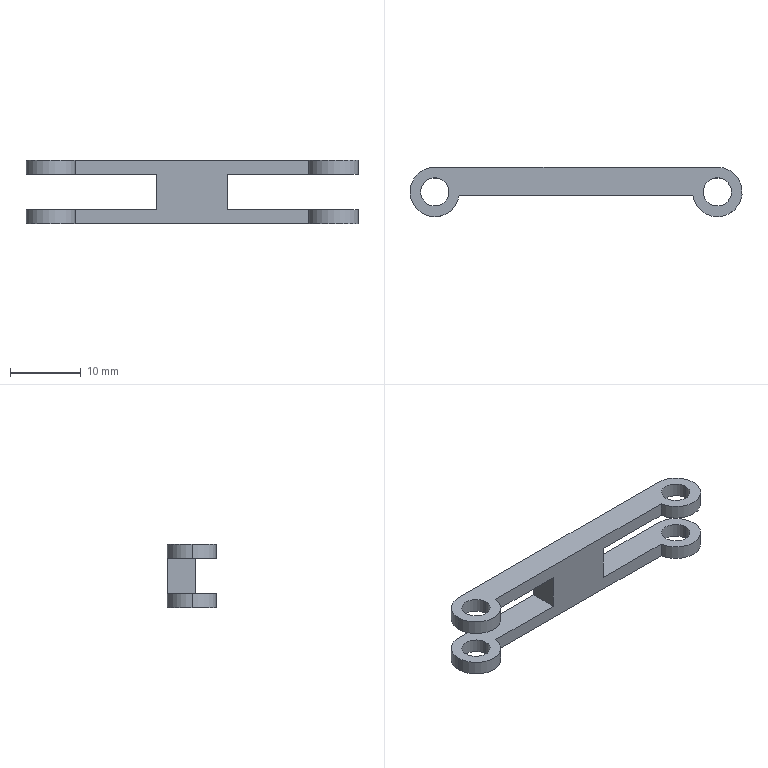Part | SolidWorks | features Extrusion 1, ICE 1, MirrorPattern 1 | 1 solid | 24 faces | box 47 x 7 x 9 mm | volume 956.424 mm3 | cylinder 14 | plane 10 | commonest cylinder face diameters 4 x8 7 x6
STEP:
#1=CARTESIAN_POINT('',(-18.,-3.5,2.));
#2=VERTEX_POINT('',#1);
#3=CARTESIAN_POINT('',(-22.,-3.5,2.));
#4=VERTEX_POINT('',#3);
#5=CARTESIAN_POINT('',(-20.,-3.5,2.));
#6=DIRECTION('',(0.,0.,-1.));
#7=DIRECTION('',(-1.,0.,0.));
#8=AXIS2_PLACEMENT_3D('',#5,#6,#7);
#9=CIRCLE('',#8,2.);
#10=EDGE_CURVE('',#2,#4,#9,.T.);
#11=ORIENTED_EDGE('',*,*,#10,.F.);
#12=CARTESIAN_POINT('',(-18.,-3.5,0.));
#13=VERTEX_POINT('',#12);
#14=CARTESIAN_POINT('',(-18.,-3.5,9.));
#15=DIRECTION('',(0.,0.,-1.));
#16=VECTOR('',#15,1000.);
#17=LINE('',#14,#16);
#18=EDGE_CURVE('',#2,#13,#17,.T.);
#19=ORIENTED_EDGE('',*,*,#18,.T.);
#20=CARTESIAN_POINT('',(-22.,-3.5,0.));
#21=VERTEX_POINT('',#20);
#22=CARTESIAN_POINT('',(-20.,-3.5,0.));
#23=DIRECTION('',(0.,0.,1.));
#24=DIRECTION('',(1.,0.,0.));
#25=AXIS2_PLACEMENT_3D('',#22,#23,#24);
#26=CIRCLE('',#25,2.);
#27=EDGE_CURVE('',#21,#13,#26,.T.);
#28=ORIENTED_EDGE('',*,*,#27,.F.);
#29=CARTESIAN_POINT('',(-22.,-3.5,9.));
#30=DIRECTION('',(0.,0.,-1.));
#31=VECTOR('',#30,1000.);
#32=LINE('',#29,#31);
#33=EDGE_CURVE('',#4,#21,#32,.T.);
#34=ORIENTED_EDGE('',*,*,#33,.F.);
#35=EDGE_LOOP('',(#11,#19,#28,#34));
#36=FACE_OUTER_BOUND('',#35,.T.);
#37=CARTESIAN_POINT('',(-20.,-3.5,9.));
#38=DIRECTION('',(0.,0.,-1.));
#39=DIRECTION('',(-1.,0.,0.));
#40=AXIS2_PLACEMENT_3D('',#37,#38,#39);
#41=CYLINDRICAL_SURFACE('',#40,2.);
#42=ADVANCED_FACE('',(#36),#41,.F.);
#43=CARTESIAN_POINT('',(-16.536,-4.,2.));
#44=VERTEX_POINT('',#43);
#45=CARTESIAN_POINT('',(-23.5,-3.5,2.));
#46=VERTEX_POINT('',#45);
#47=CARTESIAN_POINT('',(-20.,-3.5,2.));
#48=DIRECTION('',(0.,0.,-1.));
#49=DIRECTION('',(-1.,0.,0.));
#50=AXIS2_PLACEMENT_3D('',#47,#48,#49);
#51=CIRCLE('',#50,3.5);
#52=EDGE_CURVE('',#44,#46,#51,.T.);
#53=ORIENTED_EDGE('',*,*,#52,.T.);
#54=CARTESIAN_POINT('',(-23.5,-3.5,0.));
#55=VERTEX_POINT('',#54);
#56=CARTESIAN_POINT('',(-23.5,-3.5,9.));
#57=DIRECTION('',(0.,0.,-1.));
#58=VECTOR('',#57,1000.);
#59=LINE('',#56,#58);
#60=EDGE_CURVE('',#46,#55,#59,.T.);
#61=ORIENTED_EDGE('',*,*,#60,.T.);
#62=CARTESIAN_POINT('',(-16.536,-4.,0.));
#63=VERTEX_POINT('',#62);
#64=CARTESIAN_POINT('',(-20.,-3.5,0.));
#65=DIRECTION('',(0.,0.,1.));
#66=DIRECTION('',(1.,0.,0.));
#67=AXIS2_PLACEMENT_3D('',#64,#65,#66);
#68=CIRCLE('',#67,3.5);
#69=EDGE_CURVE('',#55,#63,#68,.T.);
#70=ORIENTED_EDGE('',*,*,#69,.T.);
#71=CARTESIAN_POINT('',(-16.536,-4.,9.));
#72=DIRECTION('',(0.,0.,-1.));
#73=VECTOR('',#72,1000.);
#74=LINE('',#71,#73);
#75=EDGE_CURVE('',#44,#63,#74,.T.);
#76=ORIENTED_EDGE('',*,*,#75,.F.);
#77=EDGE_LOOP('',(#53,#61,#70,#76));
#78=FACE_OUTER_BOUND('',#77,.T.);
#79=CARTESIAN_POINT('',(-20.,-3.5,9.));
#80=DIRECTION('',(0.,0.,-1.));
#81=DIRECTION('',(-1.,0.,0.));
#82=AXIS2_PLACEMENT_3D('',#79,#80,#81);
#83=CYLINDRICAL_SURFACE('',#82,3.5);
#84=ADVANCED_FACE('',(#78),#83,.T.);
#85=CARTESIAN_POINT('',(-22.,-3.5,9.));
#86=VERTEX_POINT('',#85);
#87=CARTESIAN_POINT('',(-18.,-3.5,9.));
#88=VERTEX_POINT('',#87);
#89=CARTESIAN_POINT('',(-20.,-3.5,9.));
#90=DIRECTION('',(0.,0.,1.));
#91=DIRECTION('',(1.,0.,0.));
#92=AXIS2_PLACEMENT_3D('',#89,#90,#91);
#93=CIRCLE('',#92,2.);
#94=EDGE_CURVE('',#86,#88,#93,.T.);
#95=ORIENTED_EDGE('',*,*,#94,.T.);
#96=CARTESIAN_POINT('',(-18.,-3.5,7.));
#97=VERTEX_POINT('',#96);
#98=CARTESIAN_POINT('',(-18.,-3.5,9.));
#99=DIRECTION('',(0.,0.,-1.));
#100=VECTOR('',#99,1000.);
#101=LINE('',#98,#100);
#102=EDGE_CURVE('',#88,#97,#101,.T.);
#103=ORIENTED_EDGE('',*,*,#102,.T.);
#104=CARTESIAN_POINT('',(-22.,-3.5,7.));
#105=VERTEX_POINT('',#104);
#106=CARTESIAN_POINT('',(-20.,-3.5,7.));
#107=DIRECTION('',(0.,0.,1.));
#108=DIRECTION('',(1.,0.,0.));
#109=AXIS2_PLACEMENT_3D('',#106,#107,#108);
#110=CIRCLE('',#109,2.);
#111=EDGE_CURVE('',#105,#97,#110,.T.);
#112=ORIENTED_EDGE('',*,*,#111,.F.);
#113=CARTESIAN_POINT('',(-22.,-3.5,9.));
#114=DIRECTION('',(0.,0.,-1.));
#115=VECTOR('',#114,1000.);
#116=LINE('',#113,#115);
#117=EDGE_CURVE('',#86,#105,#116,.T.);
#118=ORIENTED_EDGE('',*,*,#117,.F.);
#119=EDGE_LOOP('',(#95,#103,#112,#118));
#120=FACE_OUTER_BOUND('',#119,.T.);
#121=CARTESIAN_POINT('',(-20.,-3.5,9.));
#122=DIRECTION('',(0.,0.,-1.));
#123=DIRECTION('',(-1.,0.,0.));
#124=AXIS2_PLACEMENT_3D('',#121,#122,#123);
#125=CYLINDRICAL_SURFACE('',#124,2.);
#126=ADVANCED_FACE('',(#120),#125,.F.);
#127=CARTESIAN_POINT('',(-23.5,-3.5,9.));
#128=VERTEX_POINT('',#127);
#129=CARTESIAN_POINT('',(-16.536,-4.,9.));
#130=VERTEX_POINT('',#129);
#131=CARTESIAN_POINT('',(-20.,-3.5,9.));
#132=DIRECTION('',(0.,0.,1.));
#133=DIRECTION('',(1.,0.,0.));
#134=AXIS2_PLACEMENT_3D('',#131,#132,#133);
#135=CIRCLE('',#134,3.5);
#136=EDGE_CURVE('',#128,#130,#135,.T.);
#137=ORIENTED_EDGE('',*,*,#136,.F.);
#138=CARTESIAN_POINT('',(-23.5,-3.5,7.));
#139=VERTEX_POINT('',#138);
#140=CARTESIAN_POINT('',(-23.5,-3.5,9.));
#141=DIRECTION('',(0.,0.,-1.));
#142=VECTOR('',#141,1000.);
#143=LINE('',#140,#142);
#144=EDGE_CURVE('',#128,#139,#143,.T.);
#145=ORIENTED_EDGE('',*,*,#144,.T.);
#146=CARTESIAN_POINT('',(-16.536,-4.,7.));
#147=VERTEX_POINT('',#146);
#148=CARTESIAN_POINT('',(-20.,-3.5,7.));
#149=DIRECTION('',(0.,0.,1.));
#150=DIRECTION('',(1.,0.,0.));
#151=AXIS2_PLACEMENT_3D('',#148,#149,#150);
#152=CIRCLE('',#151,3.5);
#153=EDGE_CURVE('',#139,#147,#152,.T.);
#154=ORIENTED_EDGE('',*,*,#153,.T.);
#155=CARTESIAN_POINT('',(-16.536,-4.,9.));
#156=DIRECTION('',(0.,0.,-1.));
#157=VECTOR('',#156,1000.);
#158=LINE('',#155,#157);
#159=EDGE_CURVE('',#130,#147,#158,.T.);
#160=ORIENTED_EDGE('',*,*,#159,.F.);
#161=EDGE_LOOP('',(#137,#145,#154,#160));
#162=FACE_OUTER_BOUND('',#161,.T.);
#163=CARTESIAN_POINT('',(-20.,-3.5,9.));
#164=DIRECTION('',(0.,0.,-1.));
#165=DIRECTION('',(-1.,0.,0.));
#166=AXIS2_PLACEMENT_3D('',#163,#164,#165);
#167=CYLINDRICAL_SURFACE('',#166,3.5);
#168=ADVANCED_FACE('',(#162),#167,.T.);
#169=CARTESIAN_POINT('',(18.,-3.5,9.));
#170=VERTEX_POINT('',#169);
#171=CARTESIAN_POINT('',(22.,-3.5,9.));
#172=VERTEX_POINT('',#171);
#173=CARTESIAN_POINT('',(20.,-3.5,9.));
#174=DIRECTION('',(0.,0.,1.));
#175=DIRECTION('',(1.,0.,0.));
#176=AXIS2_PLACEMENT_3D('',#173,#174,#175);
#177=CIRCLE('',#176,2.);
#178=EDGE_CURVE('',#170,#172,#177,.T.);
#179=ORIENTED_EDGE('',*,*,#178,.T.);
#180=CARTESIAN_POINT('',(22.,-3.5,7.));
#181=VERTEX_POINT('',#180);
#182=CARTESIAN_POINT('',(22.,-3.5,9.));
#183=DIRECTION('',(0.,0.,-1.));
#184=VECTOR('',#183,1000.);
#185=LINE('',#182,#184);
#186=EDGE_CURVE('',#172,#181,#185,.T.);
#187=ORIENTED_EDGE('',*,*,#186,.T.);
#188=CARTESIAN_POINT('',(18.,-3.5,7.));
#189=VERTEX_POINT('',#188);
#190=CARTESIAN_POINT('',(20.,-3.5,7.));
#191=DIRECTION('',(0.,0.,-1.));
#192=DIRECTION('',(-1.,0.,0.));
#193=AXIS2_PLACEMENT_3D('',#190,#191,#192);
#194=CIRCLE('',#193,2.);
#195=EDGE_CURVE('',#181,#189,#194,.T.);
#196=ORIENTED_EDGE('',*,*,#195,.T.);
#197=CARTESIAN_POINT('',(18.,-3.5,9.));
#198=DIRECTION('',(0.,0.,-1.));
#199=VECTOR('',#198,1000.);
#200=LINE('',#197,#199);
#201=EDGE_CURVE('',#170,#189,#200,.T.);
#202=ORIENTED_EDGE('',*,*,#201,.F.);
#203=EDGE_LOOP('',(#179,#187,#196,#202));
#204=FACE_OUTER_BOUND('',#203,.T.);
#205=CARTESIAN_POINT('',(20.,-3.5,9.));
#206=DIRECTION('',(0.,0.,-1.));
#207=DIRECTION('',(-1.,0.,0.));
#208=AXIS2_PLACEMENT_3D('',#205,#206,#207);
#209=CYLINDRICAL_SURFACE('',#208,2.);
#210=ADVANCED_FACE('',(#204),#209,.F.);
#211=CARTESIAN_POINT('',(18.,-3.5,2.));
#212=VERTEX_POINT('',#211);
#213=CARTESIAN_POINT('',(22.,-3.5,2.));
#214=VERTEX_POINT('',#213);
#215=CARTESIAN_POINT('',(20.,-3.5,2.));
#216=DIRECTION('',(0.,0.,1.));
#217=DIRECTION('',(1.,0.,0.));
#218=AXIS2_PLACEMENT_3D('',#215,#216,#217);
#219=CIRCLE('',#218,2.);
#220=EDGE_CURVE('',#212,#214,#219,.T.);
#221=ORIENTED_EDGE('',*,*,#220,.T.);
#222=CARTESIAN_POINT('',(22.,-3.5,0.));
#223=VERTEX_POINT('',#222);
#224=CARTESIAN_POINT('',(22.,-3.5,9.));
#225=DIRECTION('',(0.,0.,-1.));
#226=VECTOR('',#225,1000.);
#227=LINE('',#224,#226);
#228=EDGE_CURVE('',#214,#223,#227,.T.);
#229=ORIENTED_EDGE('',*,*,#228,.T.);
#230=CARTESIAN_POINT('',(18.,-3.5,0.));
#231=VERTEX_POINT('',#230);
#232=CARTESIAN_POINT('',(20.,-3.5,0.));
#233=DIRECTION('',(0.,0.,1.));
#234=DIRECTION('',(1.,0.,0.));
#235=AXIS2_PLACEMENT_3D('',#232,#233,#234);
#236=CIRCLE('',#235,2.);
#237=EDGE_CURVE('',#231,#223,#236,.T.);
#238=ORIENTED_EDGE('',*,*,#237,.F.);
#239=CARTESIAN_POINT('',(18.,-3.5,9.));
#240=DIRECTION('',(0.,0.,-1.));
#241=VECTOR('',#240,1000.);
#242=LINE('',#239,#241);
#243=EDGE_CURVE('',#212,#231,#242,.T.);
#244=ORIENTED_EDGE('',*,*,#243,.F.);
#245=EDGE_LOOP('',(#221,#229,#238,#244));
#246=FACE_OUTER_BOUND('',#245,.T.);
#247=CARTESIAN_POINT('',(20.,-3.5,9.));
#248=DIRECTION('',(0.,0.,-1.));
#249=DIRECTION('',(-1.,0.,0.));
#250=AXIS2_PLACEMENT_3D('',#247,#248,#249);
#251=CYLINDRICAL_SURFACE('',#250,2.);
#252=ADVANCED_FACE('',(#246),#251,.F.);
#253=CARTESIAN_POINT('',(16.536,-4.,2.));
#254=VERTEX_POINT('',#253);
#255=CARTESIAN_POINT('',(20.,0.,2.));
#256=VERTEX_POINT('',#255);
#257=CARTESIAN_POINT('',(20.,-3.5,2.));
#258=DIRECTION('',(0.,0.,1.));
#259=DIRECTION('',(1.,0.,0.));
#260=AXIS2_PLACEMENT_3D('',#257,#258,#259);
#261=CIRCLE('',#260,3.5);
#262=EDGE_CURVE('',#254,#256,#261,.T.);
#263=ORIENTED_EDGE('',*,*,#262,.F.);
#264=CARTESIAN_POINT('',(16.536,-4.,0.));
#265=VERTEX_POINT('',#264);
#266=CARTESIAN_POINT('',(16.536,-4.,9.));
#267=DIRECTION('',(0.,0.,-1.));
#268=VECTOR('',#267,1000.);
#269=LINE('',#266,#268);
#270=EDGE_CURVE('',#254,#265,#269,.T.);
#271=ORIENTED_EDGE('',*,*,#270,.T.);
#272=CARTESIAN_POINT('',(20.,0.,0.));
#273=VERTEX_POINT('',#272);
#274=CARTESIAN_POINT('',(20.,-3.5,0.));
#275=DIRECTION('',(0.,0.,1.));
#276=DIRECTION('',(1.,0.,0.));
#277=AXIS2_PLACEMENT_3D('',#274,#275,#276);
#278=CIRCLE('',#277,3.5);
#279=EDGE_CURVE('',#265,#273,#278,.T.);
#280=ORIENTED_EDGE('',*,*,#279,.T.);
#281=CARTESIAN_POINT('',(20.,0.,9.));
#282=DIRECTION('',(0.,0.,-1.));
#283=VECTOR('',#282,1000.);
#284=LINE('',#281,#283);
#285=EDGE_CURVE('',#256,#273,#284,.T.);
#286=ORIENTED_EDGE('',*,*,#285,.F.);
#287=EDGE_LOOP('',(#263,#271,#280,#286));
#288=FACE_OUTER_BOUND('',#287,.T.);
#289=CARTESIAN_POINT('',(20.,-3.5,9.));
#290=DIRECTION('',(0.,0.,-1.));
#291=DIRECTION('',(-1.,0.,0.));
#292=AXIS2_PLACEMENT_3D('',#289,#290,#291);
#293=CYLINDRICAL_SURFACE('',#292,3.5);
#294=ADVANCED_FACE('',(#288),#293,.T.);
#295=CARTESIAN_POINT('',(20.,0.,7.));
#296=VERTEX_POINT('',#295);
#297=CARTESIAN_POINT('',(16.536,-4.,7.));
#298=VERTEX_POINT('',#297);
#299=CARTESIAN_POINT('',(20.,-3.5,7.));
#300=DIRECTION('',(0.,0.,-1.));
#301=DIRECTION('',(-1.,0.,0.));
#302=AXIS2_PLACEMENT_3D('',#299,#300,#301);
#303=CIRCLE('',#302,3.5);
#304=EDGE_CURVE('',#296,#298,#303,.T.);
#305=ORIENTED_EDGE('',*,*,#304,.F.);
#306=CARTESIAN_POINT('',(20.,0.,9.));
#307=VERTEX_POINT('',#306);
#308=CARTESIAN_POINT('',(20.,0.,9.));
#309=DIRECTION('',(0.,0.,-1.));
#310=VECTOR('',#309,1000.);
#311=LINE('',#308,#310);
#312=EDGE_CURVE('',#307,#296,#311,.T.);
#313=ORIENTED_EDGE('',*,*,#312,.F.);
#314=CARTESIAN_POINT('',(16.536,-4.,9.));
#315=VERTEX_POINT('',#314);
#316=CARTESIAN_POINT('',(20.,-3.5,9.));
#317=DIRECTION('',(0.,0.,1.));
#318=DIRECTION('',(1.,0.,0.));
#319=AXIS2_PLACEMENT_3D('',#316,#317,#318);
#320=CIRCLE('',#319,3.5);
#321=EDGE_CURVE('',#315,#307,#320,.T.);
#322=ORIENTED_EDGE('',*,*,#321,.F.);
#323=CARTESIAN_POINT('',(16.536,-4.,9.));
#324=DIRECTION('',(0.,0.,-1.));
#325=VECTOR('',#324,1000.);
#326=LINE('',#323,#325);
#327=EDGE_CURVE('',#315,#298,#326,.T.);
#328=ORIENTED_EDGE('',*,*,#327,.T.);
#329=EDGE_LOOP('',(#305,#313,#322,#328));
#330=FACE_OUTER_BOUND('',#329,.T.);
#331=CARTESIAN_POINT('',(20.,-3.5,9.));
#332=DIRECTION('',(0.,0.,-1.));
#333=DIRECTION('',(-1.,0.,0.));
#334=AXIS2_PLACEMENT_3D('',#331,#332,#333);
#335=CYLINDRICAL_SURFACE('',#334,3.5);
#336=ADVANCED_FACE('',(#330),#335,.T.);
#337=CARTESIAN_POINT('',(5.,0.,2.));
#338=VERTEX_POINT('',#337);
#339=CARTESIAN_POINT('',(42.,0.,2.));
#340=DIRECTION('',(1.,0.,0.));
#341=VECTOR('',#340,1000.);
#342=LINE('',#339,#341);
#343=EDGE_CURVE('',#338,#256,#342,.T.);
#344=ORIENTED_EDGE('',*,*,#343,.T.);
#345=ORIENTED_EDGE('',*,*,#285,.T.);
#346=CARTESIAN_POINT('',(-20.,0.,0.));
#347=VERTEX_POINT('',#346);
#348=CARTESIAN_POINT('',(-20.,0.,0.));
#349=DIRECTION('',(-1.,0.,0.));
#350=VECTOR('',#349,1000.);
#351=LINE('',#348,#350);
#352=EDGE_CURVE('',#273,#347,#351,.T.);
#353=ORIENTED_EDGE('',*,*,#352,.T.);
#354=CARTESIAN_POINT('',(-20.,0.,2.));
#355=VERTEX_POINT('',#354);
#356=CARTESIAN_POINT('',(-20.,0.,9.));
#357=DIRECTION('',(0.,0.,-1.));
#358=VECTOR('',#357,1000.);
#359=LINE('',#356,#358);
#360=EDGE_CURVE('',#355,#347,#359,.T.);
#361=ORIENTED_EDGE('',*,*,#360,.F.);
#362=CARTESIAN_POINT('',(-5.,0.,2.));
#363=VERTEX_POINT('',#362);
#364=CARTESIAN_POINT('',(-42.,0.,2.));
#365=DIRECTION('',(-1.,0.,0.));
#366=VECTOR('',#365,1000.);
#367=LINE('',#364,#366);
#368=EDGE_CURVE('',#363,#355,#367,.T.);
#369=ORIENTED_EDGE('',*,*,#368,.F.);
#370=CARTESIAN_POINT('',(-5.,0.,7.));
#371=VERTEX_POINT('',#370);
#372=CARTESIAN_POINT('',(-5.,0.,2.));
#373=DIRECTION('',(0.,0.,-1.));
#374=VECTOR('',#373,1000.);
#375=LINE('',#372,#374);
#376=EDGE_CURVE('',#371,#363,#375,.T.);
#377=ORIENTED_EDGE('',*,*,#376,.F.);
#378=CARTESIAN_POINT('',(-20.,0.,7.));
#379=VERTEX_POINT('',#378);
#380=CARTESIAN_POINT('',(-42.,0.,7.));
#381=DIRECTION('',(1.,0.,0.));
#382=VECTOR('',#381,1000.);
#383=LINE('',#380,#382);
#384=EDGE_CURVE('',#379,#371,#383,.T.);
#385=ORIENTED_EDGE('',*,*,#384,.F.);
#386=CARTESIAN_POINT('',(-20.,0.,9.));
#387=VERTEX_POINT('',#386);
#388=CARTESIAN_POINT('',(-20.,0.,9.));
#389=DIRECTION('',(0.,0.,-1.));
#390=VECTOR('',#389,1000.);
#391=LINE('',#388,#390);
#392=EDGE_CURVE('',#387,#379,#391,.T.);
#393=ORIENTED_EDGE('',*,*,#392,.F.);
#394=CARTESIAN_POINT('',(-20.,0.,9.));
#395=DIRECTION('',(-1.,0.,0.));
#396=VECTOR('',#395,1000.);
#397=LINE('',#394,#396);
#398=EDGE_CURVE('',#307,#387,#397,.T.);
#399=ORIENTED_EDGE('',*,*,#398,.F.);
#400=ORIENTED_EDGE('',*,*,#312,.T.);
#401=CARTESIAN_POINT('',(5.,0.,7.));
#402=VERTEX_POINT('',#401);
#403=CARTESIAN_POINT('',(42.,0.,7.));
#404=DIRECTION('',(-1.,0.,0.));
#405=VECTOR('',#404,1000.);
#406=LINE('',#403,#405);
#407=EDGE_CURVE('',#296,#402,#406,.T.);
#408=ORIENTED_EDGE('',*,*,#407,.T.);
#409=CARTESIAN_POINT('',(5.,0.,2.));
#410=DIRECTION('',(0.,0.,-1.));
#411=VECTOR('',#410,1000.);
#412=LINE('',#409,#411);
#413=EDGE_CURVE('',#402,#338,#412,.T.);
#414=ORIENTED_EDGE('',*,*,#413,.T.);
#415=EDGE_LOOP('',(#344,#345,#353,#361,#369,#377,#385,#393,#399,#400,#408,#414));
#416=FACE_OUTER_BOUND('',#415,.T.);
#417=CARTESIAN_POINT('',(-20.,0.,9.));
#418=DIRECTION('',(0.,-1.,0.));
#419=DIRECTION('',(0.,0.,-1.));
#420=AXIS2_PLACEMENT_3D('',#417,#418,#419);
#421=PLANE('',#420);
#422=ADVANCED_FACE('',(#416),#421,.F.);
#423=CARTESIAN_POINT('',(5.,-4.,2.));
#424=VERTEX_POINT('',#423);
#425=CARTESIAN_POINT('',(-16.536,-4.,2.));
#426=DIRECTION('',(1.,0.,0.));
#427=VECTOR('',#426,1000.);
#428=LINE('',#425,#427);
#429=EDGE_CURVE('',#424,#254,#428,.T.);
#430=ORIENTED_EDGE('',*,*,#429,.F.);
#431=CARTESIAN_POINT('',(5.,-4.,7.));
#432=VERTEX_POINT('',#431);
#433=CARTESIAN_POINT('',(5.,-4.,9.));
#434=DIRECTION('',(0.,0.,-1.));
#435=VECTOR('',#434,1000.);
#436=LINE('',#433,#435);
#437=EDGE_CURVE('',#432,#424,#436,.T.);
#438=ORIENTED_EDGE('',*,*,#437,.F.);
#439=CARTESIAN_POINT('',(-16.536,-4.,7.));
#440=DIRECTION('',(-1.,0.,0.));
#441=VECTOR('',#440,1000.);
#442=LINE('',#439,#441);
#443=EDGE_CURVE('',#298,#432,#442,.T.);
#444=ORIENTED_EDGE('',*,*,#443,.F.);
#445=ORIENTED_EDGE('',*,*,#327,.F.);
#446=CARTESIAN_POINT('',(-16.536,-4.,9.));
#447=DIRECTION('',(1.,0.,0.));
#448=VECTOR('',#447,1000.);
#449=LINE('',#446,#448);
#450=EDGE_CURVE('',#130,#315,#449,.T.);
#451=ORIENTED_EDGE('',*,*,#450,.F.);
#452=ORIENTED_EDGE('',*,*,#159,.T.);
#453=CARTESIAN_POINT('',(-5.,-4.,7.));
#454=VERTEX_POINT('',#453);
#455=CARTESIAN_POINT('',(-16.536,-4.,7.));
#456=DIRECTION('',(1.,0.,0.));
#457=VECTOR('',#456,1000.);
#458=LINE('',#455,#457);
#459=EDGE_CURVE('',#147,#454,#458,.T.);
#460=ORIENTED_EDGE('',*,*,#459,.T.);
#461=CARTESIAN_POINT('',(-5.,-4.,2.));
#462=VERTEX_POINT('',#461);
#463=CARTESIAN_POINT('',(-5.,-4.,9.));
#464=DIRECTION('',(0.,0.,-1.));
#465=VECTOR('',#464,1000.);
#466=LINE('',#463,#465);
#467=EDGE_CURVE('',#454,#462,#466,.T.);
#468=ORIENTED_EDGE('',*,*,#467,.T.);
#469=CARTESIAN_POINT('',(-16.536,-4.,2.));
#470=DIRECTION('',(-1.,0.,0.));
#471=VECTOR('',#470,1000.);
#472=LINE('',#469,#471);
#473=EDGE_CURVE('',#462,#44,#472,.T.);
#474=ORIENTED_EDGE('',*,*,#473,.T.);
#475=ORIENTED_EDGE('',*,*,#75,.T.);
#476=CARTESIAN_POINT('',(-16.536,-4.,0.));
#477=DIRECTION('',(1.,0.,0.));
#478=VECTOR('',#477,1000.);
#479=LINE('',#476,#478);
#480=EDGE_CURVE('',#63,#265,#479,.T.);
#481=ORIENTED_EDGE('',*,*,#480,.T.);
#482=ORIENTED_EDGE('',*,*,#270,.F.);
#483=EDGE_LOOP('',(#430,#438,#444,#445,#451,#452,#460,#468,#474,#475,#481,#482));
#484=FACE_OUTER_BOUND('',#483,.T.);
#485=CARTESIAN_POINT('',(-16.536,-4.,9.));
#486=DIRECTION('',(0.,1.,0.));
#487=DIRECTION('',(0.,0.,1.));
#488=AXIS2_PLACEMENT_3D('',#485,#486,#487);
#489=PLANE('',#488);
#490=ADVANCED_FACE('',(#484),#489,.F.);
#491=ORIENTED_EDGE('',*,*,#228,.F.);
#492=CARTESIAN_POINT('',(20.,-3.5,2.));
#493=DIRECTION('',(0.,0.,1.));
#494=DIRECTION('',(1.,0.,0.));
#495=AXIS2_PLACEMENT_3D('',#492,#493,#494);
#496=CIRCLE('',#495,2.);
#497=EDGE_CURVE('',#214,#212,#496,.T.);
#498=ORIENTED_EDGE('',*,*,#497,.T.);
#499=ORIENTED_EDGE('',*,*,#243,.T.);
#500=CARTESIAN_POINT('',(20.,-3.5,0.));
#501=DIRECTION('',(0.,0.,1.));
#502=DIRECTION('',(1.,0.,0.));
#503=AXIS2_PLACEMENT_3D('',#500,#501,#502);
#504=CIRCLE('',#503,2.);
#505=EDGE_CURVE('',#223,#231,#504,.T.);
#506=ORIENTED_EDGE('',*,*,#505,.F.);
#507=EDGE_LOOP('',(#491,#498,#499,#506));
#508=FACE_OUTER_BOUND('',#507,.T.);
#509=CARTESIAN_POINT('',(20.,-3.5,9.));
#510=DIRECTION('',(0.,0.,-1.));
#511=DIRECTION('',(-1.,0.,0.));
#512=AXIS2_PLACEMENT_3D('',#509,#510,#511);
#513=CYLINDRICAL_SURFACE('',#512,2.);
#514=ADVANCED_FACE('',(#508),#513,.F.);
#515=ORIENTED_EDGE('',*,*,#186,.F.);
#516=CARTESIAN_POINT('',(20.,-3.5,9.));
#517=DIRECTION('',(0.,0.,1.));
#518=DIRECTION('',(1.,0.,0.));
#519=AXIS2_PLACEMENT_3D('',#516,#517,#518);
#520=CIRCLE('',#519,2.);
#521=EDGE_CURVE('',#172,#170,#520,.T.);
#522=ORIENTED_EDGE('',*,*,#521,.T.);
#523=ORIENTED_EDGE('',*,*,#201,.T.);
#524=CARTESIAN_POINT('',(20.,-3.5,7.));
#525=DIRECTION('',(0.,0.,-1.));
#526=DIRECTION('',(-1.,0.,0.));
#527=AXIS2_PLACEMENT_3D('',#524,#525,#526);
#528=CIRCLE('',#527,2.);
#529=EDGE_CURVE('',#189,#181,#528,.T.);
#530=ORIENTED_EDGE('',*,*,#529,.T.);
#531=EDGE_LOOP('',(#515,#522,#523,#530));
#532=FACE_OUTER_BOUND('',#531,.T.);
#533=CARTESIAN_POINT('',(20.,-3.5,9.));
#534=DIRECTION('',(0.,0.,-1.));
#535=DIRECTION('',(-1.,0.,0.));
#536=AXIS2_PLACEMENT_3D('',#533,#534,#535);
#537=CYLINDRICAL_SURFACE('',#536,2.);
#538=ADVANCED_FACE('',(#532),#537,.F.);
#539=ORIENTED_EDGE('',*,*,#144,.F.);
#540=CARTESIAN_POINT('',(-20.,-3.5,9.));
#541=DIRECTION('',(0.,0.,1.));
#542=DIRECTION('',(1.,0.,0.));
#543=AXIS2_PLACEMENT_3D('',#540,#541,#542);
#544=CIRCLE('',#543,3.5);
#545=EDGE_CURVE('',#387,#128,#544,.T.);
#546=ORIENTED_EDGE('',*,*,#545,.F.);
#547=ORIENTED_EDGE('',*,*,#392,.T.);
#548=CARTESIAN_POINT('',(-20.,-3.5,7.));
#549=DIRECTION('',(0.,0.,1.));
#550=DIRECTION('',(1.,0.,0.));
#551=AXIS2_PLACEMENT_3D('',#548,#549,#550);
#552=CIRCLE('',#551,3.5);
#553=EDGE_CURVE('',#379,#139,#552,.T.);
#554=ORIENTED_EDGE('',*,*,#553,.T.);
#555=EDGE_LOOP('',(#539,#546,#547,#554));
#556=FACE_OUTER_BOUND('',#555,.T.);
#557=CARTESIAN_POINT('',(-20.,-3.5,9.));
#558=DIRECTION('',(0.,0.,-1.));
#559=DIRECTION('',(-1.,0.,0.));
#560=AXIS2_PLACEMENT_3D('',#557,#558,#559);
#561=CYLINDRICAL_SURFACE('',#560,3.5);
#562=ADVANCED_FACE('',(#556),#561,.T.);
#563=ORIENTED_EDGE('',*,*,#102,.F.);
#564=CARTESIAN_POINT('',(-20.,-3.5,9.));
#565=DIRECTION('',(0.,0.,1.));
#566=DIRECTION('',(1.,0.,0.));
#567=AXIS2_PLACEMENT_3D('',#564,#565,#566);
#568=CIRCLE('',#567,2.);
#569=EDGE_CURVE('',#88,#86,#568,.T.);
#570=ORIENTED_EDGE('',*,*,#569,.T.);
#571=ORIENTED_EDGE('',*,*,#117,.T.);
#572=CARTESIAN_POINT('',(-20.,-3.5,7.));
#573=DIRECTION('',(0.,0.,1.));
#574=DIRECTION('',(1.,0.,0.));
#575=AXIS2_PLACEMENT_3D('',#572,#573,#574);
#576=CIRCLE('',#575,2.);
#577=EDGE_CURVE('',#97,#105,#576,.T.);
#578=ORIENTED_EDGE('',*,*,#577,.F.);
#579=EDGE_LOOP('',(#563,#570,#571,#578));
#580=FACE_OUTER_BOUND('',#579,.T.);
#581=CARTESIAN_POINT('',(-20.,-3.5,9.));
#582=DIRECTION('',(0.,0.,-1.));
#583=DIRECTION('',(-1.,0.,0.));
#584=AXIS2_PLACEMENT_3D('',#581,#582,#583);
#585=CYLINDRICAL_SURFACE('',#584,2.);
#586=ADVANCED_FACE('',(#580),#585,.F.);
#587=ORIENTED_EDGE('',*,*,#178,.F.);
#588=ORIENTED_EDGE('',*,*,#521,.F.);
#589=EDGE_LOOP('',(#587,#588));
#590=FACE_BOUND('',#589,.T.);
#591=ORIENTED_EDGE('',*,*,#321,.T.);
#592=ORIENTED_EDGE('',*,*,#398,.T.);
#593=ORIENTED_EDGE('',*,*,#545,.T.);
#594=ORIENTED_EDGE('',*,*,#136,.T.);
#595=ORIENTED_EDGE('',*,*,#450,.T.);
#596=EDGE_LOOP('',(#591,#592,#593,#594,#595));
#597=FACE_OUTER_BOUND('',#596,.T.);
#598=ORIENTED_EDGE('',*,*,#94,.F.);
#599=ORIENTED_EDGE('',*,*,#569,.F.);
#600=EDGE_LOOP('',(#598,#599));
#601=FACE_BOUND('',#600,.T.);
#602=CARTESIAN_POINT('',(20.,-3.5,9.));
#603=DIRECTION('',(0.,0.,1.));
#604=DIRECTION('',(1.,0.,0.));
#605=AXIS2_PLACEMENT_3D('',#602,#603,#604);
#606=PLANE('',#605);
#607=ADVANCED_FACE('',(#590,#597,#601),#606,.T.);
#608=ORIENTED_EDGE('',*,*,#279,.F.);
#609=ORIENTED_EDGE('',*,*,#480,.F.);
#610=ORIENTED_EDGE('',*,*,#69,.F.);
#611=CARTESIAN_POINT('',(-20.,-3.5,0.));
#612=DIRECTION('',(0.,0.,1.));
#613=DIRECTION('',(1.,0.,0.));
#614=AXIS2_PLACEMENT_3D('',#611,#612,#613);
#615=CIRCLE('',#614,3.5);
#616=EDGE_CURVE('',#347,#55,#615,.T.);
#617=ORIENTED_EDGE('',*,*,#616,.F.);
#618=ORIENTED_EDGE('',*,*,#352,.F.);
#619=EDGE_LOOP('',(#608,#609,#610,#617,#618));
#620=FACE_OUTER_BOUND('',#619,.T.);
#621=ORIENTED_EDGE('',*,*,#237,.T.);
#622=ORIENTED_EDGE('',*,*,#505,.T.);
#623=EDGE_LOOP('',(#621,#622));
#624=FACE_BOUND('',#623,.T.);
#625=ORIENTED_EDGE('',*,*,#27,.T.);
#626=CARTESIAN_POINT('',(-20.,-3.5,0.));
#627=DIRECTION('',(0.,0.,1.));
#628=DIRECTION('',(1.,0.,0.));
#629=AXIS2_PLACEMENT_3D('',#626,#627,#628);
#630=CIRCLE('',#629,2.);
#631=EDGE_CURVE('',#13,#21,#630,.T.);
#632=ORIENTED_EDGE('',*,*,#631,.T.);
#633=EDGE_LOOP('',(#625,#632));
#634=FACE_BOUND('',#633,.T.);
#635=CARTESIAN_POINT('',(20.,-3.5,0.));
#636=DIRECTION('',(0.,0.,1.));
#637=DIRECTION('',(1.,0.,0.));
#638=AXIS2_PLACEMENT_3D('',#635,#636,#637);
#639=PLANE('',#638);
#640=ADVANCED_FACE('',(#620,#624,#634),#639,.F.);
#641=ORIENTED_EDGE('',*,*,#60,.F.);
#642=CARTESIAN_POINT('',(-20.,-3.5,2.));
#643=DIRECTION('',(0.,0.,-1.));
#644=DIRECTION('',(-1.,0.,0.));
#645=AXIS2_PLACEMENT_3D('',#642,#643,#644);
#646=CIRCLE('',#645,3.5);
#647=EDGE_CURVE('',#46,#355,#646,.T.);
#648=ORIENTED_EDGE('',*,*,#647,.T.);
#649=ORIENTED_EDGE('',*,*,#360,.T.);
#650=ORIENTED_EDGE('',*,*,#616,.T.);
#651=EDGE_LOOP('',(#641,#648,#649,#650));
#652=FACE_OUTER_BOUND('',#651,.T.);
#653=CARTESIAN_POINT('',(-20.,-3.5,9.));
#654=DIRECTION('',(0.,0.,-1.));
#655=DIRECTION('',(-1.,0.,0.));
#656=AXIS2_PLACEMENT_3D('',#653,#654,#655);
#657=CYLINDRICAL_SURFACE('',#656,3.5);
#658=ADVANCED_FACE('',(#652),#657,.T.);
#659=ORIENTED_EDGE('',*,*,#18,.F.);
#660=CARTESIAN_POINT('',(-20.,-3.5,2.));
#661=DIRECTION('',(0.,0.,-1.));
#662=DIRECTION('',(-1.,0.,0.));
#663=AXIS2_PLACEMENT_3D('',#660,#661,#662);
#664=CIRCLE('',#663,2.);
#665=EDGE_CURVE('',#4,#2,#664,.T.);
#666=ORIENTED_EDGE('',*,*,#665,.F.);
#667=ORIENTED_EDGE('',*,*,#33,.T.);
#668=ORIENTED_EDGE('',*,*,#631,.F.);
#669=EDGE_LOOP('',(#659,#666,#667,#668));
#670=FACE_OUTER_BOUND('',#669,.T.);
#671=CARTESIAN_POINT('',(-20.,-3.5,9.));
#672=DIRECTION('',(0.,0.,-1.));
#673=DIRECTION('',(-1.,0.,0.));
#674=AXIS2_PLACEMENT_3D('',#671,#672,#673);
#675=CYLINDRICAL_SURFACE('',#674,2.);
#676=ADVANCED_FACE('',(#670),#675,.F.);
#677=CARTESIAN_POINT('',(-5.,-9.,7.));
#678=DIRECTION('',(0.,1.,0.));
#679=VECTOR('',#678,1000.);
#680=LINE('',#677,#679);
#681=EDGE_CURVE('',#454,#371,#680,.T.);
#682=ORIENTED_EDGE('',*,*,#681,.T.);
#683=ORIENTED_EDGE('',*,*,#376,.T.);
#684=CARTESIAN_POINT('',(-5.,-9.,2.));
#685=DIRECTION('',(0.,1.,0.));
#686=VECTOR('',#685,1000.);
#687=LINE('',#684,#686);
#688=EDGE_CURVE('',#462,#363,#687,.T.);
#689=ORIENTED_EDGE('',*,*,#688,.F.);
#690=ORIENTED_EDGE('',*,*,#467,.F.);
#691=EDGE_LOOP('',(#682,#683,#689,#690));
#692=FACE_OUTER_BOUND('',#691,.T.);
#693=CARTESIAN_POINT('',(-5.,-9.,2.));
#694=DIRECTION('',(1.,0.,0.));
#695=DIRECTION('',(0.,0.,-1.));
#696=AXIS2_PLACEMENT_3D('',#693,#694,#695);
#697=PLANE('',#696);
#698=ADVANCED_FACE('',(#692),#697,.F.);
#699=ORIENTED_EDGE('',*,*,#111,.T.);
#700=ORIENTED_EDGE('',*,*,#577,.T.);
#701=EDGE_LOOP('',(#699,#700));
#702=FACE_BOUND('',#701,.T.);
#703=ORIENTED_EDGE('',*,*,#384,.T.);
#704=ORIENTED_EDGE('',*,*,#681,.F.);
#705=ORIENTED_EDGE('',*,*,#459,.F.);
#706=ORIENTED_EDGE('',*,*,#153,.F.);
#707=ORIENTED_EDGE('',*,*,#553,.F.);
#708=EDGE_LOOP('',(#703,#704,#705,#706,#707));
#709=FACE_OUTER_BOUND('',#708,.T.);
#710=CARTESIAN_POINT('',(-42.,-9.,7.));
#711=DIRECTION('',(0.,0.,1.));
#712=DIRECTION('',(1.,0.,0.));
#713=AXIS2_PLACEMENT_3D('',#710,#711,#712);
#714=PLANE('',#713);
#715=ADVANCED_FACE('',(#702,#709),#714,.F.);
#716=ORIENTED_EDGE('',*,*,#665,.T.);
#717=ORIENTED_EDGE('',*,*,#10,.T.);
#718=EDGE_LOOP('',(#716,#717));
#719=FACE_BOUND('',#718,.T.);
#720=ORIENTED_EDGE('',*,*,#473,.F.);
#721=ORIENTED_EDGE('',*,*,#688,.T.);
#722=ORIENTED_EDGE('',*,*,#368,.T.);
#723=ORIENTED_EDGE('',*,*,#647,.F.);
#724=ORIENTED_EDGE('',*,*,#52,.F.);
#725=EDGE_LOOP('',(#720,#721,#722,#723,#724));
#726=FACE_OUTER_BOUND('',#725,.T.);
#727=CARTESIAN_POINT('',(-42.,-9.,2.));
#728=DIRECTION('',(0.,0.,-1.));
#729=DIRECTION('',(-1.,0.,0.));
#730=AXIS2_PLACEMENT_3D('',#727,#728,#729);
#731=PLANE('',#730);
#732=ADVANCED_FACE('',(#719,#726),#731,.F.);
#733=ORIENTED_EDGE('',*,*,#437,.T.);
#734=CARTESIAN_POINT('',(5.,-9.,2.));
#735=DIRECTION('',(0.,1.,0.));
#736=VECTOR('',#735,1000.);
#737=LINE('',#734,#736);
#738=EDGE_CURVE('',#424,#338,#737,.T.);
#739=ORIENTED_EDGE('',*,*,#738,.T.);
#740=ORIENTED_EDGE('',*,*,#413,.F.);
#741=CARTESIAN_POINT('',(5.,-9.,7.));
#742=DIRECTION('',(0.,1.,0.));
#743=VECTOR('',#742,1000.);
#744=LINE('',#741,#743);
#745=EDGE_CURVE('',#432,#402,#744,.T.);
#746=ORIENTED_EDGE('',*,*,#745,.F.);
#747=EDGE_LOOP('',(#733,#739,#740,#746));
#748=FACE_OUTER_BOUND('',#747,.T.);
#749=CARTESIAN_POINT('',(5.,-9.,2.));
#750=DIRECTION('',(1.,0.,0.));
#751=DIRECTION('',(0.,0.,-1.));
#752=AXIS2_PLACEMENT_3D('',#749,#750,#751);
#753=PLANE('',#752);
#754=ADVANCED_FACE('',(#748),#753,.T.);
#755=ORIENTED_EDGE('',*,*,#220,.F.);
#756=ORIENTED_EDGE('',*,*,#497,.F.);
#757=EDGE_LOOP('',(#755,#756));
#758=FACE_BOUND('',#757,.T.);
#759=ORIENTED_EDGE('',*,*,#262,.T.);
#760=ORIENTED_EDGE('',*,*,#343,.F.);
#761=ORIENTED_EDGE('',*,*,#738,.F.);
#762=ORIENTED_EDGE('',*,*,#429,.T.);
#763=EDGE_LOOP('',(#759,#760,#761,#762));
#764=FACE_OUTER_BOUND('',#763,.T.);
#765=CARTESIAN_POINT('',(42.,-9.,2.));
#766=DIRECTION('',(0.,0.,1.));
#767=DIRECTION('',(1.,0.,0.));
#768=AXIS2_PLACEMENT_3D('',#765,#766,#767);
#769=PLANE('',#768);
#770=ADVANCED_FACE('',(#758,#764),#769,.T.);
#771=ORIENTED_EDGE('',*,*,#529,.F.);
#772=ORIENTED_EDGE('',*,*,#195,.F.);
#773=EDGE_LOOP('',(#771,#772));
#774=FACE_BOUND('',#773,.T.);
#775=ORIENTED_EDGE('',*,*,#304,.T.);
#776=ORIENTED_EDGE('',*,*,#443,.T.);
#777=ORIENTED_EDGE('',*,*,#745,.T.);
#778=ORIENTED_EDGE('',*,*,#407,.F.);
#779=EDGE_LOOP('',(#775,#776,#777,#778));
#780=FACE_OUTER_BOUND('',#779,.T.);
#781=CARTESIAN_POINT('',(42.,-9.,7.));
#782=DIRECTION('',(0.,0.,-1.));
#783=DIRECTION('',(-1.,0.,0.));
#784=AXIS2_PLACEMENT_3D('',#781,#782,#783);
#785=PLANE('',#784);
#786=ADVANCED_FACE('',(#774,#780),#785,.T.);
#787=CLOSED_SHELL('',(#42,#84,#126,#168,#210,#252,#294,#336,#422,#490,#514,#538,#562,#586,#607,#640,#658,#676,#698,#715,#732,#754,#770,#786));
#788=MANIFOLD_SOLID_BREP('',#787);
#789=CARTESIAN_POINT('',(0.,0.,0.));
#790=DIRECTION('',(0.,0.,1.));
#791=DIRECTION('',(1.,0.,0.));
#792=AXIS2_PLACEMENT_3D('',#789,#790,#791);
#793=(LENGTH_UNIT()NAMED_UNIT(*)SI_UNIT(.MILLI.,.METRE.));
#794=UNCERTAINTY_MEASURE_WITH_UNIT(LENGTH_MEASURE(0.00001),#793,'','');
#795=(NAMED_UNIT(*)PLANE_ANGLE_UNIT()SI_UNIT($,.RADIAN.));
#796=(NAMED_UNIT(*)SI_UNIT($,.STERADIAN.)SOLID_ANGLE_UNIT());
#797=(GEOMETRIC_REPRESENTATION_CONTEXT(3)GLOBAL_UNCERTAINTY_ASSIGNED_CONTEXT((#794))GLOBAL_UNIT_ASSIGNED_CONTEXT((#793,#795,#796))REPRESENTATION_CONTEXT('',''));
#798=ADVANCED_BREP_SHAPE_REPRESENTATION('',(#788,#792),#797);